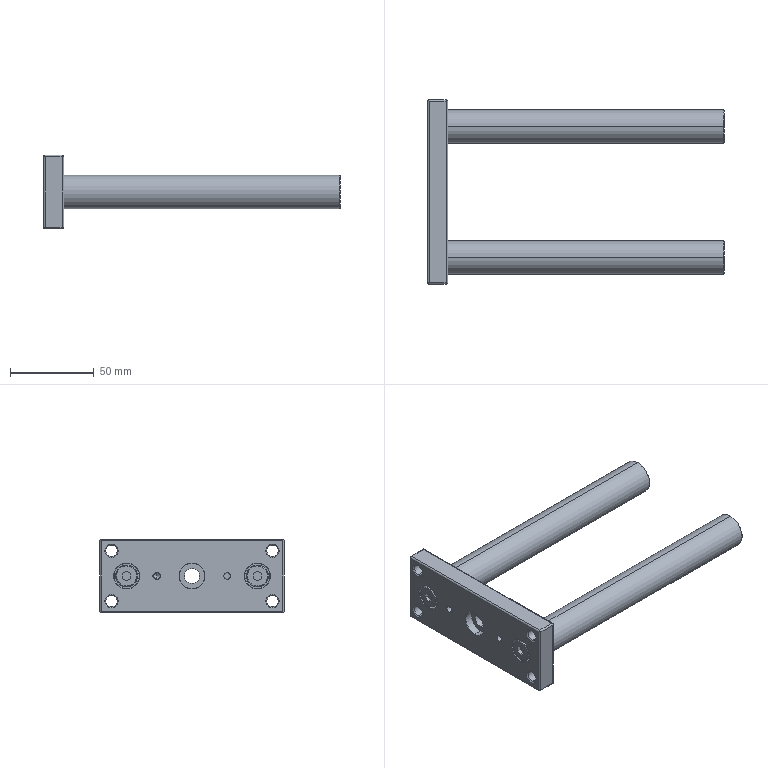Part | SolidWorks | features BaseBody 1 | 1 solid | 106 faces | box 177 x 110 x 44 mm | volume 157829 mm3 | cylinder 42 | plane 32 | cone 28 | spline 4 | commonest cylinder face diameters 2 x12 6.647 x8 4 x6 15 x6 13 x4 20 x4